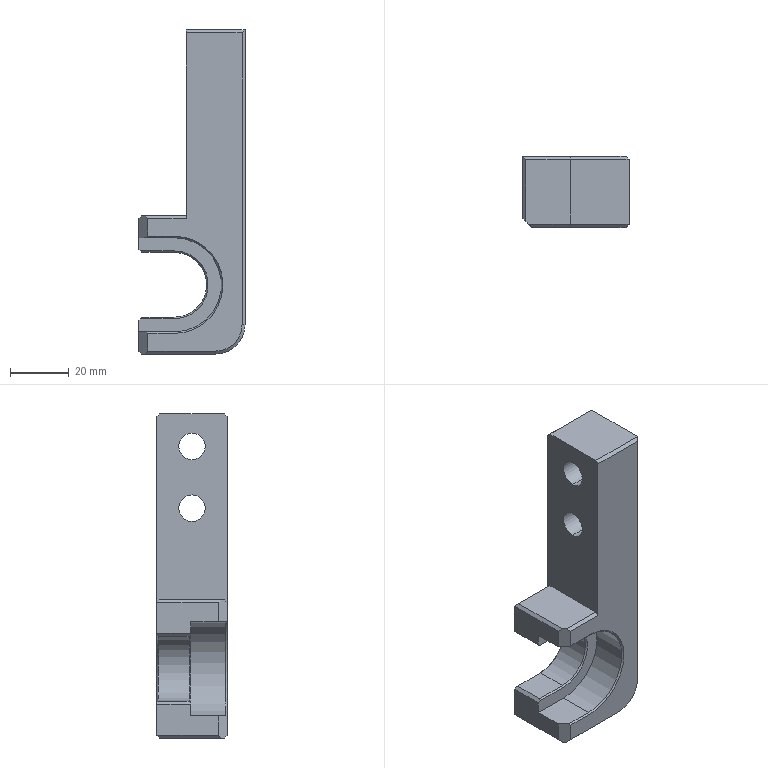Part | SolidWorks | features Chamfer 7, ICE 3, Extrusion 1, Fillet 1, HoleWzd 1 | 1 solid | 52 faces | box 36 x 24 x 110 mm | volume 50408 mm3 | plane 36 | cylinder 11 | cone 5 | commonest cylinder face diameters 9 x4 15 x4 20 x1 22 x1 32 x1
STEP:
#1=CARTESIAN_POINT('',(1.,0.,325.519));
#2=VERTEX_POINT('',#1);
#3=CARTESIAN_POINT('',(1.,0.,310.519));
#4=VERTEX_POINT('',#3);
#5=CARTESIAN_POINT('',(1.,0.,318.019));
#6=DIRECTION('',(1.,0.,0.));
#7=DIRECTION('',(0.,0.,-1.));
#8=AXIS2_PLACEMENT_3D('',#5,#6,#7);
#9=CIRCLE('',#8,7.5);
#10=EDGE_CURVE('',#2,#4,#9,.T.);
#11=ORIENTED_EDGE('',*,*,#10,.F.);
#12=CARTESIAN_POINT('',(10.,0.,325.519));
#13=VERTEX_POINT('',#12);
#14=CARTESIAN_POINT('',(10.,0.,325.519));
#15=DIRECTION('',(1.,0.,0.));
#16=VECTOR('',#15,1000.);
#17=LINE('',#14,#16);
#18=EDGE_CURVE('',#2,#13,#17,.T.);
#19=ORIENTED_EDGE('',*,*,#18,.T.);
#20=CARTESIAN_POINT('',(10.,0.,310.519));
#21=VERTEX_POINT('',#20);
#22=CARTESIAN_POINT('',(10.,0.,318.019));
#23=DIRECTION('',(1.,0.,0.));
#24=DIRECTION('',(0.,0.,-1.));
#25=AXIS2_PLACEMENT_3D('',#22,#23,#24);
#26=CIRCLE('',#25,7.5);
#27=EDGE_CURVE('',#13,#21,#26,.T.);
#28=ORIENTED_EDGE('',*,*,#27,.T.);
#29=CARTESIAN_POINT('',(10.,0.,310.519));
#30=DIRECTION('',(1.,0.,0.));
#31=VECTOR('',#30,1000.);
#32=LINE('',#29,#31);
#33=EDGE_CURVE('',#4,#21,#32,.T.);
#34=ORIENTED_EDGE('',*,*,#33,.F.);
#35=EDGE_LOOP('',(#11,#19,#28,#34));
#36=FACE_OUTER_BOUND('',#35,.T.);
#37=CARTESIAN_POINT('',(10.,0.,318.019));
#38=DIRECTION('',(1.,0.,0.));
#39=DIRECTION('',(0.,0.,-1.));
#40=AXIS2_PLACEMENT_3D('',#37,#38,#39);
#41=CYLINDRICAL_SURFACE('',#40,7.5);
#42=ADVANCED_FACE('',(#36),#41,.F.);
#43=CARTESIAN_POINT('',(-10.,0.,322.519));
#44=VERTEX_POINT('',#43);
#45=CARTESIAN_POINT('',(-10.,0.,313.519));
#46=VERTEX_POINT('',#45);
#47=CARTESIAN_POINT('',(-10.,0.,318.019));
#48=DIRECTION('',(1.,0.,0.));
#49=DIRECTION('',(0.,1.,0.));
#50=AXIS2_PLACEMENT_3D('',#47,#48,#49);
#51=CIRCLE('',#50,4.5);
#52=EDGE_CURVE('',#44,#46,#51,.T.);
#53=ORIENTED_EDGE('',*,*,#52,.F.);
#54=CARTESIAN_POINT('',(1.,0.,322.519));
#55=VERTEX_POINT('',#54);
#56=CARTESIAN_POINT('',(10.,0.,322.519));
#57=DIRECTION('',(1.,0.,0.));
#58=VECTOR('',#57,1000.);
#59=LINE('',#56,#58);
#60=EDGE_CURVE('',#44,#55,#59,.T.);
#61=ORIENTED_EDGE('',*,*,#60,.T.);
#62=CARTESIAN_POINT('',(1.,0.,313.519));
#63=VERTEX_POINT('',#62);
#64=CARTESIAN_POINT('',(1.,0.,318.019));
#65=DIRECTION('',(1.,0.,0.));
#66=DIRECTION('',(0.,0.,-1.));
#67=AXIS2_PLACEMENT_3D('',#64,#65,#66);
#68=CIRCLE('',#67,4.5);
#69=EDGE_CURVE('',#55,#63,#68,.T.);
#70=ORIENTED_EDGE('',*,*,#69,.T.);
#71=CARTESIAN_POINT('',(10.,0.,313.519));
#72=DIRECTION('',(1.,0.,0.));
#73=VECTOR('',#72,1000.);
#74=LINE('',#71,#73);
#75=EDGE_CURVE('',#46,#63,#74,.T.);
#76=ORIENTED_EDGE('',*,*,#75,.F.);
#77=EDGE_LOOP('',(#53,#61,#70,#76));
#78=FACE_OUTER_BOUND('',#77,.T.);
#79=CARTESIAN_POINT('',(10.,0.,318.019));
#80=DIRECTION('',(1.,0.,0.));
#81=DIRECTION('',(0.,0.,-1.));
#82=AXIS2_PLACEMENT_3D('',#79,#80,#81);
#83=CYLINDRICAL_SURFACE('',#82,4.5);
#84=ADVANCED_FACE('',(#78),#83,.F.);
#85=CARTESIAN_POINT('',(1.,0.,304.519));
#86=VERTEX_POINT('',#85);
#87=CARTESIAN_POINT('',(1.,0.,289.519));
#88=VERTEX_POINT('',#87);
#89=CARTESIAN_POINT('',(1.,0.,297.019));
#90=DIRECTION('',(1.,0.,0.));
#91=DIRECTION('',(0.,0.,-1.));
#92=AXIS2_PLACEMENT_3D('',#89,#90,#91);
#93=CIRCLE('',#92,7.5);
#94=EDGE_CURVE('',#86,#88,#93,.T.);
#95=ORIENTED_EDGE('',*,*,#94,.F.);
#96=CARTESIAN_POINT('',(10.,0.,304.519));
#97=VERTEX_POINT('',#96);
#98=CARTESIAN_POINT('',(10.,0.,304.519));
#99=DIRECTION('',(1.,0.,0.));
#100=VECTOR('',#99,1000.);
#101=LINE('',#98,#100);
#102=EDGE_CURVE('',#86,#97,#101,.T.);
#103=ORIENTED_EDGE('',*,*,#102,.T.);
#104=CARTESIAN_POINT('',(10.,0.,289.519));
#105=VERTEX_POINT('',#104);
#106=CARTESIAN_POINT('',(10.,0.,297.019));
#107=DIRECTION('',(1.,0.,0.));
#108=DIRECTION('',(0.,0.,-1.));
#109=AXIS2_PLACEMENT_3D('',#106,#107,#108);
#110=CIRCLE('',#109,7.5);
#111=EDGE_CURVE('',#97,#105,#110,.T.);
#112=ORIENTED_EDGE('',*,*,#111,.T.);
#113=CARTESIAN_POINT('',(10.,0.,289.519));
#114=DIRECTION('',(1.,0.,0.));
#115=VECTOR('',#114,1000.);
#116=LINE('',#113,#115);
#117=EDGE_CURVE('',#88,#105,#116,.T.);
#118=ORIENTED_EDGE('',*,*,#117,.F.);
#119=EDGE_LOOP('',(#95,#103,#112,#118));
#120=FACE_OUTER_BOUND('',#119,.T.);
#121=CARTESIAN_POINT('',(10.,0.,297.019));
#122=DIRECTION('',(1.,0.,0.));
#123=DIRECTION('',(0.,0.,-1.));
#124=AXIS2_PLACEMENT_3D('',#121,#122,#123);
#125=CYLINDRICAL_SURFACE('',#124,7.5);
#126=ADVANCED_FACE('',(#120),#125,.F.);
#127=CARTESIAN_POINT('',(-10.,0.,301.519));
#128=VERTEX_POINT('',#127);
#129=CARTESIAN_POINT('',(-10.,0.,292.519));
#130=VERTEX_POINT('',#129);
#131=CARTESIAN_POINT('',(-10.,0.,297.019));
#132=DIRECTION('',(1.,0.,0.));
#133=DIRECTION('',(0.,1.,0.));
#134=AXIS2_PLACEMENT_3D('',#131,#132,#133);
#135=CIRCLE('',#134,4.5);
#136=EDGE_CURVE('',#128,#130,#135,.T.);
#137=ORIENTED_EDGE('',*,*,#136,.F.);
#138=CARTESIAN_POINT('',(1.,0.,301.519));
#139=VERTEX_POINT('',#138);
#140=CARTESIAN_POINT('',(10.,0.,301.519));
#141=DIRECTION('',(1.,0.,0.));
#142=VECTOR('',#141,1000.);
#143=LINE('',#140,#142);
#144=EDGE_CURVE('',#128,#139,#143,.T.);
#145=ORIENTED_EDGE('',*,*,#144,.T.);
#146=CARTESIAN_POINT('',(1.,0.,292.519));
#147=VERTEX_POINT('',#146);
#148=CARTESIAN_POINT('',(1.,0.,297.019));
#149=DIRECTION('',(1.,0.,0.));
#150=DIRECTION('',(0.,0.,-1.));
#151=AXIS2_PLACEMENT_3D('',#148,#149,#150);
#152=CIRCLE('',#151,4.5);
#153=EDGE_CURVE('',#139,#147,#152,.T.);
#154=ORIENTED_EDGE('',*,*,#153,.T.);
#155=CARTESIAN_POINT('',(10.,0.,292.519));
#156=DIRECTION('',(1.,0.,0.));
#157=VECTOR('',#156,1000.);
#158=LINE('',#155,#157);
#159=EDGE_CURVE('',#130,#147,#158,.T.);
#160=ORIENTED_EDGE('',*,*,#159,.F.);
#161=EDGE_LOOP('',(#137,#145,#154,#160));
#162=FACE_OUTER_BOUND('',#161,.T.);
#163=CARTESIAN_POINT('',(10.,0.,297.019));
#164=DIRECTION('',(1.,0.,0.));
#165=DIRECTION('',(0.,0.,-1.));
#166=AXIS2_PLACEMENT_3D('',#163,#164,#165);
#167=CYLINDRICAL_SURFACE('',#166,4.5);
#168=ADVANCED_FACE('',(#162),#167,.F.);
#169=CARTESIAN_POINT('',(-26.,-9.,258.519));
#170=VERTEX_POINT('',#169);
#171=CARTESIAN_POINT('',(-26.,0.5,258.519));
#172=VERTEX_POINT('',#171);
#173=CARTESIAN_POINT('',(-26.,0.,258.519));
#174=DIRECTION('',(0.,1.,0.));
#175=VECTOR('',#174,1000.);
#176=LINE('',#173,#175);
#177=EDGE_CURVE('',#170,#172,#176,.T.);
#178=ORIENTED_EDGE('',*,*,#177,.F.);
#179=CARTESIAN_POINT('',(-26.,-9.,265.019));
#180=VERTEX_POINT('',#179);
#181=CARTESIAN_POINT('',(-26.,-9.,0.));
#182=DIRECTION('',(0.,0.,1.));
#183=VECTOR('',#182,1000.);
#184=LINE('',#181,#183);
#185=EDGE_CURVE('',#170,#180,#184,.T.);
#186=ORIENTED_EDGE('',*,*,#185,.T.);
#187=CARTESIAN_POINT('',(-26.,12.,265.019));
#188=VERTEX_POINT('',#187);
#189=CARTESIAN_POINT('',(-26.,0.,265.019));
#190=DIRECTION('',(0.,1.,0.));
#191=VECTOR('',#190,1000.);
#192=LINE('',#189,#191);
#193=EDGE_CURVE('',#180,#188,#192,.T.);
#194=ORIENTED_EDGE('',*,*,#193,.T.);
#195=CARTESIAN_POINT('',(-26.,12.,254.519));
#196=VERTEX_POINT('',#195);
#197=CARTESIAN_POINT('',(-26.,12.,219.019));
#198=DIRECTION('',(0.,0.,-1.));
#199=VECTOR('',#198,1000.);
#200=LINE('',#197,#199);
#201=EDGE_CURVE('',#188,#196,#200,.T.);
#202=ORIENTED_EDGE('',*,*,#201,.T.);
#203=CARTESIAN_POINT('',(-26.,0.5,254.519));
#204=VERTEX_POINT('',#203);
#205=CARTESIAN_POINT('',(-26.,0.,254.519));
#206=DIRECTION('',(0.,-1.,0.));
#207=VECTOR('',#206,1000.);
#208=LINE('',#205,#207);
#209=EDGE_CURVE('',#196,#204,#208,.T.);
#210=ORIENTED_EDGE('',*,*,#209,.T.);
#211=CARTESIAN_POINT('',(-26.,0.5,0.));
#212=DIRECTION('',(0.,0.,1.));
#213=VECTOR('',#212,1000.);
#214=LINE('',#211,#213);
#215=EDGE_CURVE('',#204,#172,#214,.T.);
#216=ORIENTED_EDGE('',*,*,#215,.T.);
#217=EDGE_LOOP('',(#178,#186,#194,#202,#210,#216));
#218=FACE_OUTER_BOUND('',#217,.T.);
#219=CARTESIAN_POINT('',(-26.,0.,0.));
#220=DIRECTION('',(1.,0.,0.));
#221=DIRECTION('',(0.,1.,0.));
#222=AXIS2_PLACEMENT_3D('',#219,#220,#221);
#223=PLANE('',#222);
#224=ADVANCED_FACE('',(#218),#223,.F.);
#225=CARTESIAN_POINT('',(-14.,-12.,226.019));
#226=VERTEX_POINT('',#225);
#227=CARTESIAN_POINT('',(-23.,-12.,226.019));
#228=VERTEX_POINT('',#227);
#229=CARTESIAN_POINT('',(-26.,-12.,226.019));
#230=DIRECTION('',(-1.,0.,0.));
#231=VECTOR('',#230,1000.);
#232=LINE('',#229,#231);
#233=EDGE_CURVE('',#226,#228,#232,.T.);
#234=ORIENTED_EDGE('',*,*,#233,.T.);
#235=CARTESIAN_POINT('',(-23.,-12.,220.019));
#236=VERTEX_POINT('',#235);
#237=CARTESIAN_POINT('',(-23.,-12.,329.019));
#238=DIRECTION('',(0.,0.,-1.));
#239=VECTOR('',#238,1000.);
#240=LINE('',#237,#239);
#241=EDGE_CURVE('',#228,#236,#240,.T.);
#242=ORIENTED_EDGE('',*,*,#241,.T.);
#243=CARTESIAN_POINT('',(0.,-12.,220.019));
#244=VERTEX_POINT('',#243);
#245=CARTESIAN_POINT('',(-10.,-12.,220.019));
#246=DIRECTION('',(1.,0.,0.));
#247=VECTOR('',#246,1000.);
#248=LINE('',#245,#247);
#249=EDGE_CURVE('',#236,#244,#248,.T.);
#250=ORIENTED_EDGE('',*,*,#249,.T.);
#251=CARTESIAN_POINT('',(9.,-12.,229.019));
#252=VERTEX_POINT('',#251);
#253=CARTESIAN_POINT('',(0.,-12.,229.019));
#254=DIRECTION('',(0.,-1.,0.));
#255=DIRECTION('',(0.,0.,1.));
#256=AXIS2_PLACEMENT_3D('',#253,#254,#255);
#257=CIRCLE('',#256,9.);
#258=EDGE_CURVE('',#244,#252,#257,.T.);
#259=ORIENTED_EDGE('',*,*,#258,.T.);
#260=CARTESIAN_POINT('',(9.,-12.,328.019));
#261=VERTEX_POINT('',#260);
#262=CARTESIAN_POINT('',(9.,-12.,329.019));
#263=DIRECTION('',(0.,0.,1.));
#264=VECTOR('',#263,1000.);
#265=LINE('',#262,#264);
#266=EDGE_CURVE('',#252,#261,#265,.T.);
#267=ORIENTED_EDGE('',*,*,#266,.T.);
#268=CARTESIAN_POINT('',(-10.,-12.,328.019));
#269=VERTEX_POINT('',#268);
#270=CARTESIAN_POINT('',(-10.,-12.,328.019));
#271=DIRECTION('',(-1.,0.,0.));
#272=VECTOR('',#271,1000.);
#273=LINE('',#270,#272);
#274=EDGE_CURVE('',#261,#269,#273,.T.);
#275=ORIENTED_EDGE('',*,*,#274,.T.);
#276=CARTESIAN_POINT('',(-10.,-12.,265.019));
#277=VERTEX_POINT('',#276);
#278=CARTESIAN_POINT('',(-10.,-12.,329.019));
#279=DIRECTION('',(0.,0.,-1.));
#280=VECTOR('',#279,1000.);
#281=LINE('',#278,#280);
#282=EDGE_CURVE('',#269,#277,#281,.T.);
#283=ORIENTED_EDGE('',*,*,#282,.T.);
#284=CARTESIAN_POINT('',(-23.,-12.,265.019));
#285=VERTEX_POINT('',#284);
#286=CARTESIAN_POINT('',(-10.,-12.,265.019));
#287=DIRECTION('',(-1.,0.,0.));
#288=VECTOR('',#287,1000.);
#289=LINE('',#286,#288);
#290=EDGE_CURVE('',#277,#285,#289,.T.);
#291=ORIENTED_EDGE('',*,*,#290,.T.);
#292=CARTESIAN_POINT('',(-23.,-12.,259.019));
#293=VERTEX_POINT('',#292);
#294=CARTESIAN_POINT('',(-23.,-12.,329.019));
#295=DIRECTION('',(0.,0.,-1.));
#296=VECTOR('',#295,1000.);
#297=LINE('',#294,#296);
#298=EDGE_CURVE('',#285,#293,#297,.T.);
#299=ORIENTED_EDGE('',*,*,#298,.T.);
#300=CARTESIAN_POINT('',(-14.,-12.,259.019));
#301=VERTEX_POINT('',#300);
#302=CARTESIAN_POINT('',(-14.,-12.,259.019));
#303=DIRECTION('',(1.,0.,0.));
#304=VECTOR('',#303,1000.);
#305=LINE('',#302,#304);
#306=EDGE_CURVE('',#293,#301,#305,.T.);
#307=ORIENTED_EDGE('',*,*,#306,.T.);
#308=CARTESIAN_POINT('',(-14.,-12.,242.519));
#309=DIRECTION('',(0.,1.,0.));
#310=DIRECTION('',(0.,0.,1.));
#311=AXIS2_PLACEMENT_3D('',#308,#309,#310);
#312=CIRCLE('',#311,16.5);
#313=EDGE_CURVE('',#301,#226,#312,.T.);
#314=ORIENTED_EDGE('',*,*,#313,.T.);
#315=EDGE_LOOP('',(#234,#242,#250,#259,#267,#275,#283,#291,#299,#307,#314));
#316=FACE_OUTER_BOUND('',#315,.T.);
#317=CARTESIAN_POINT('',(-10.,-12.,329.019));
#318=DIRECTION('',(0.,1.,0.));
#319=DIRECTION('',(0.,0.,1.));
#320=AXIS2_PLACEMENT_3D('',#317,#318,#319);
#321=PLANE('',#320);
#322=ADVANCED_FACE('',(#316),#321,.F.);
#323=CARTESIAN_POINT('',(-26.,12.,220.019));
#324=VERTEX_POINT('',#323);
#325=CARTESIAN_POINT('',(-26.,-9.,220.019));
#326=VERTEX_POINT('',#325);
#327=CARTESIAN_POINT('',(-26.,0.,220.019));
#328=DIRECTION('',(0.,-1.,0.));
#329=VECTOR('',#328,1000.);
#330=LINE('',#327,#329);
#331=EDGE_CURVE('',#324,#326,#330,.T.);
#332=ORIENTED_EDGE('',*,*,#331,.T.);
#333=CARTESIAN_POINT('',(-26.,-9.,226.519));
#334=VERTEX_POINT('',#333);
#335=CARTESIAN_POINT('',(-26.,-9.,0.));
#336=DIRECTION('',(0.,0.,1.));
#337=VECTOR('',#336,1000.);
#338=LINE('',#335,#337);
#339=EDGE_CURVE('',#326,#334,#338,.T.);
#340=ORIENTED_EDGE('',*,*,#339,.T.);
#341=CARTESIAN_POINT('',(-26.,0.5,226.519));
#342=VERTEX_POINT('',#341);
#343=CARTESIAN_POINT('',(-26.,0.,226.519));
#344=DIRECTION('',(0.,-1.,0.));
#345=VECTOR('',#344,1000.);
#346=LINE('',#343,#345);
#347=EDGE_CURVE('',#342,#334,#346,.T.);
#348=ORIENTED_EDGE('',*,*,#347,.F.);
#349=CARTESIAN_POINT('',(-26.,0.5,230.519));
#350=VERTEX_POINT('',#349);
#351=CARTESIAN_POINT('',(-26.,0.5,0.));
#352=DIRECTION('',(0.,0.,1.));
#353=VECTOR('',#352,1000.);
#354=LINE('',#351,#353);
#355=EDGE_CURVE('',#342,#350,#354,.T.);
#356=ORIENTED_EDGE('',*,*,#355,.T.);
#357=CARTESIAN_POINT('',(-26.,12.,230.519));
#358=VERTEX_POINT('',#357);
#359=CARTESIAN_POINT('',(-26.,0.,230.519));
#360=DIRECTION('',(0.,1.,0.));
#361=VECTOR('',#360,1000.);
#362=LINE('',#359,#361);
#363=EDGE_CURVE('',#350,#358,#362,.T.);
#364=ORIENTED_EDGE('',*,*,#363,.T.);
#365=CARTESIAN_POINT('',(-26.,12.,219.019));
#366=DIRECTION('',(0.,0.,-1.));
#367=VECTOR('',#366,1000.);
#368=LINE('',#365,#367);
#369=EDGE_CURVE('',#358,#324,#368,.T.);
#370=ORIENTED_EDGE('',*,*,#369,.T.);
#371=EDGE_LOOP('',(#332,#340,#348,#356,#364,#370));
#372=FACE_OUTER_BOUND('',#371,.T.);
#373=CARTESIAN_POINT('',(-26.,0.,0.));
#374=DIRECTION('',(1.,0.,0.));
#375=DIRECTION('',(0.,1.,0.));
#376=AXIS2_PLACEMENT_3D('',#373,#374,#375);
#377=PLANE('',#376);
#378=ADVANCED_FACE('',(#372),#377,.F.);
#379=CARTESIAN_POINT('',(-10.,0.,318.019));
#380=DIRECTION('',(1.,0.,0.));
#381=DIRECTION('',(0.,1.,0.));
#382=AXIS2_PLACEMENT_3D('',#379,#380,#381);
#383=CIRCLE('',#382,4.5);
#384=EDGE_CURVE('',#46,#44,#383,.T.);
#385=ORIENTED_EDGE('',*,*,#384,.T.);
#386=ORIENTED_EDGE('',*,*,#52,.T.);
#387=EDGE_LOOP('',(#385,#386));
#388=FACE_BOUND('',#387,.T.);
#389=CARTESIAN_POINT('',(-10.,0.,297.019));
#390=DIRECTION('',(1.,0.,0.));
#391=DIRECTION('',(0.,1.,0.));
#392=AXIS2_PLACEMENT_3D('',#389,#390,#391);
#393=CIRCLE('',#392,4.5);
#394=EDGE_CURVE('',#130,#128,#393,.T.);
#395=ORIENTED_EDGE('',*,*,#394,.T.);
#396=ORIENTED_EDGE('',*,*,#136,.T.);
#397=EDGE_LOOP('',(#395,#396));
#398=FACE_BOUND('',#397,.T.);
#399=CARTESIAN_POINT('',(-10.,11.,329.019));
#400=VERTEX_POINT('',#399);
#401=CARTESIAN_POINT('',(-10.,-11.,329.019));
#402=VERTEX_POINT('',#401);
#403=CARTESIAN_POINT('',(-10.,12.,329.019));
#404=DIRECTION('',(0.,-1.,0.));
#405=VECTOR('',#404,1000.);
#406=LINE('',#403,#405);
#407=EDGE_CURVE('',#400,#402,#406,.T.);
#408=ORIENTED_EDGE('',*,*,#407,.F.);
#409=CARTESIAN_POINT('',(-10.,12.,328.019));
#410=VERTEX_POINT('',#409);
#411=CARTESIAN_POINT('',(-10.,11.,329.019));
#412=DIRECTION('',(0.,0.7071,-0.7071));
#413=VECTOR('',#412,1000.);
#414=LINE('',#411,#413);
#415=EDGE_CURVE('',#400,#410,#414,.T.);
#416=ORIENTED_EDGE('',*,*,#415,.T.);
#417=CARTESIAN_POINT('',(-10.,12.,265.019));
#418=VERTEX_POINT('',#417);
#419=CARTESIAN_POINT('',(-10.,12.,329.019));
#420=DIRECTION('',(0.,0.,-1.));
#421=VECTOR('',#420,1000.);
#422=LINE('',#419,#421);
#423=EDGE_CURVE('',#410,#418,#422,.T.);
#424=ORIENTED_EDGE('',*,*,#423,.T.);
#425=CARTESIAN_POINT('',(-10.,11.,266.019));
#426=VERTEX_POINT('',#425);
#427=CARTESIAN_POINT('',(-10.,-20.,297.019));
#428=DIRECTION('',(0.,-0.7071,0.7071));
#429=VECTOR('',#428,1000.);
#430=LINE('',#427,#429);
#431=EDGE_CURVE('',#418,#426,#430,.T.);
#432=ORIENTED_EDGE('',*,*,#431,.T.);
#433=CARTESIAN_POINT('',(-10.,-11.,266.019));
#434=VERTEX_POINT('',#433);
#435=CARTESIAN_POINT('',(-10.,-12.,266.019));
#436=DIRECTION('',(0.,1.,0.));
#437=VECTOR('',#436,1000.);
#438=LINE('',#435,#437);
#439=EDGE_CURVE('',#434,#426,#438,.T.);
#440=ORIENTED_EDGE('',*,*,#439,.F.);
#441=CARTESIAN_POINT('',(-10.,32.,309.019));
#442=DIRECTION('',(0.,-0.7071,-0.7071));
#443=VECTOR('',#442,1000.);
#444=LINE('',#441,#443);
#445=EDGE_CURVE('',#434,#277,#444,.T.);
#446=ORIENTED_EDGE('',*,*,#445,.T.);
#447=ORIENTED_EDGE('',*,*,#282,.F.);
#448=CARTESIAN_POINT('',(-10.,-11.,329.019));
#449=DIRECTION('',(0.,0.7071,0.7071));
#450=VECTOR('',#449,1000.);
#451=LINE('',#448,#450);
#452=EDGE_CURVE('',#269,#402,#451,.T.);
#453=ORIENTED_EDGE('',*,*,#452,.T.);
#454=EDGE_LOOP('',(#408,#416,#424,#432,#440,#446,#447,#453));
#455=FACE_OUTER_BOUND('',#454,.T.);
#456=CARTESIAN_POINT('',(-10.,12.,329.019));
#457=DIRECTION('',(1.,0.,0.));
#458=DIRECTION('',(0.,1.,0.));
#459=AXIS2_PLACEMENT_3D('',#456,#457,#458);
#460=PLANE('',#459);
#461=ADVANCED_FACE('',(#388,#398,#455),#460,.F.);
#462=CARTESIAN_POINT('',(10.,0.,318.019));
#463=DIRECTION('',(1.,0.,0.));
#464=DIRECTION('',(0.,0.,-1.));
#465=AXIS2_PLACEMENT_3D('',#462,#463,#464);
#466=CIRCLE('',#465,7.5);
#467=EDGE_CURVE('',#21,#13,#466,.T.);
#468=ORIENTED_EDGE('',*,*,#467,.F.);
#469=ORIENTED_EDGE('',*,*,#27,.F.);
#470=EDGE_LOOP('',(#468,#469));
#471=FACE_BOUND('',#470,.T.);
#472=CARTESIAN_POINT('',(10.,0.,297.019));
#473=DIRECTION('',(1.,0.,0.));
#474=DIRECTION('',(0.,0.,-1.));
#475=AXIS2_PLACEMENT_3D('',#472,#473,#474);
#476=CIRCLE('',#475,7.5);
#477=EDGE_CURVE('',#105,#97,#476,.T.);
#478=ORIENTED_EDGE('',*,*,#477,.F.);
#479=ORIENTED_EDGE('',*,*,#111,.F.);
#480=EDGE_LOOP('',(#478,#479));
#481=FACE_BOUND('',#480,.T.);
#482=CARTESIAN_POINT('',(10.,-11.,229.019));
#483=VERTEX_POINT('',#482);
#484=CARTESIAN_POINT('',(10.,11.,229.019));
#485=VERTEX_POINT('',#484);
#486=CARTESIAN_POINT('',(10.,12.,229.019));
#487=DIRECTION('',(0.,1.,0.));
#488=VECTOR('',#487,1000.);
#489=LINE('',#486,#488);
#490=EDGE_CURVE('',#483,#485,#489,.T.);
#491=ORIENTED_EDGE('',*,*,#490,.T.);
#492=CARTESIAN_POINT('',(10.,11.,329.019));
#493=VERTEX_POINT('',#492);
#494=CARTESIAN_POINT('',(10.,11.,329.019));
#495=DIRECTION('',(0.,0.,1.));
#496=VECTOR('',#495,1000.);
#497=LINE('',#494,#496);
#498=EDGE_CURVE('',#485,#493,#497,.T.);
#499=ORIENTED_EDGE('',*,*,#498,.T.);
#500=CARTESIAN_POINT('',(10.,-11.,329.019));
#501=VERTEX_POINT('',#500);
#502=CARTESIAN_POINT('',(10.,12.,329.019));
#503=DIRECTION('',(0.,1.,0.));
#504=VECTOR('',#503,1000.);
#505=LINE('',#502,#504);
#506=EDGE_CURVE('',#501,#493,#505,.T.);
#507=ORIENTED_EDGE('',*,*,#506,.F.);
#508=CARTESIAN_POINT('',(10.,-11.,329.019));
#509=DIRECTION('',(0.,0.,-1.));
#510=VECTOR('',#509,1000.);
#511=LINE('',#508,#510);
#512=EDGE_CURVE('',#501,#483,#511,.T.);
#513=ORIENTED_EDGE('',*,*,#512,.T.);
#514=EDGE_LOOP('',(#491,#499,#507,#513));
#515=FACE_OUTER_BOUND('',#514,.T.);
#516=CARTESIAN_POINT('',(10.,12.,329.019));
#517=DIRECTION('',(-1.,0.,0.));
#518=DIRECTION('',(0.,-1.,0.));
#519=AXIS2_PLACEMENT_3D('',#516,#517,#518);
#520=PLANE('',#519);
#521=ADVANCED_FACE('',(#471,#481,#515),#520,.F.);
#522=ORIENTED_EDGE('',*,*,#201,.F.);
#523=CARTESIAN_POINT('',(-10.,12.,265.019));
#524=DIRECTION('',(1.,0.,0.));
#525=VECTOR('',#524,1000.);
#526=LINE('',#523,#525);
#527=EDGE_CURVE('',#188,#418,#526,.T.);
#528=ORIENTED_EDGE('',*,*,#527,.T.);
#529=ORIENTED_EDGE('',*,*,#423,.F.);
#530=CARTESIAN_POINT('',(9.,12.,328.019));
#531=VERTEX_POINT('',#530);
#532=CARTESIAN_POINT('',(10.,12.,328.019));
#533=DIRECTION('',(1.,0.,0.));
#534=VECTOR('',#533,1000.);
#535=LINE('',#532,#534);
#536=EDGE_CURVE('',#410,#531,#535,.T.);
#537=ORIENTED_EDGE('',*,*,#536,.T.);
#538=CARTESIAN_POINT('',(9.,12.,229.019));
#539=VERTEX_POINT('',#538);
#540=CARTESIAN_POINT('',(9.,12.,329.019));
#541=DIRECTION('',(0.,0.,-1.));
#542=VECTOR('',#541,1000.);
#543=LINE('',#540,#542);
#544=EDGE_CURVE('',#531,#539,#543,.T.);
#545=ORIENTED_EDGE('',*,*,#544,.T.);
#546=CARTESIAN_POINT('',(0.,12.,220.019));
#547=VERTEX_POINT('',#546);
#548=CARTESIAN_POINT('',(0.,12.,229.019));
#549=DIRECTION('',(0.,1.,0.));
#550=DIRECTION('',(0.,0.,-1.));
#551=AXIS2_PLACEMENT_3D('',#548,#549,#550);
#552=CIRCLE('',#551,9.);
#553=EDGE_CURVE('',#539,#547,#552,.T.);
#554=ORIENTED_EDGE('',*,*,#553,.T.);
#555=CARTESIAN_POINT('',(-10.,12.,220.019));
#556=DIRECTION('',(-1.,0.,0.));
#557=VECTOR('',#556,1000.);
#558=LINE('',#555,#557);
#559=EDGE_CURVE('',#547,#324,#558,.T.);
#560=ORIENTED_EDGE('',*,*,#559,.T.);
#561=ORIENTED_EDGE('',*,*,#369,.F.);
#562=CARTESIAN_POINT('',(-25.5,12.,231.019));
#563=VERTEX_POINT('',#562);
#564=CARTESIAN_POINT('',(-26.,12.,230.519));
#565=DIRECTION('',(0.7071,0.,0.7071));
#566=VECTOR('',#565,1000.);
#567=LINE('',#564,#566);
#568=EDGE_CURVE('',#358,#563,#567,.T.);
#569=ORIENTED_EDGE('',*,*,#568,.T.);
#570=CARTESIAN_POINT('',(-14.,12.,231.019));
#571=VERTEX_POINT('',#570);
#572=CARTESIAN_POINT('',(-10.,12.,231.019));
#573=DIRECTION('',(1.,0.,0.));
#574=VECTOR('',#573,1000.);
#575=LINE('',#572,#574);
#576=EDGE_CURVE('',#563,#571,#575,.T.);
#577=ORIENTED_EDGE('',*,*,#576,.T.);
#578=CARTESIAN_POINT('',(-14.,12.,254.019));
#579=VERTEX_POINT('',#578);
#580=CARTESIAN_POINT('',(-14.,12.,242.519));
#581=DIRECTION('',(0.,-1.,0.));
#582=DIRECTION('',(0.,0.,-1.));
#583=AXIS2_PLACEMENT_3D('',#580,#581,#582);
#584=CIRCLE('',#583,11.5);
#585=EDGE_CURVE('',#571,#579,#584,.T.);
#586=ORIENTED_EDGE('',*,*,#585,.T.);
#587=CARTESIAN_POINT('',(-25.5,12.,254.019));
#588=VERTEX_POINT('',#587);
#589=CARTESIAN_POINT('',(-10.,12.,254.019));
#590=DIRECTION('',(-1.,0.,0.));
#591=VECTOR('',#590,1000.);
#592=LINE('',#589,#591);
#593=EDGE_CURVE('',#579,#588,#592,.T.);
#594=ORIENTED_EDGE('',*,*,#593,.T.);
#595=CARTESIAN_POINT('',(-26.,12.,254.519));
#596=DIRECTION('',(-0.7071,0.,0.7071));
#597=VECTOR('',#596,1000.);
#598=LINE('',#595,#597);
#599=EDGE_CURVE('',#588,#196,#598,.T.);
#600=ORIENTED_EDGE('',*,*,#599,.T.);
#601=EDGE_LOOP('',(#522,#528,#529,#537,#545,#554,#560,#561,#569,#577,#586,#594,#600));
#602=FACE_OUTER_BOUND('',#601,.T.);
#603=CARTESIAN_POINT('',(-10.,12.,329.019));
#604=DIRECTION('',(0.,-1.,0.));
#605=DIRECTION('',(0.,0.,-1.));
#606=AXIS2_PLACEMENT_3D('',#603,#604,#605);
#607=PLANE('',#606);
#608=ADVANCED_FACE('',(#602),#607,.F.);
#609=ORIENTED_EDGE('',*,*,#506,.T.);
#610=CARTESIAN_POINT('',(-10.,11.,329.019));
#611=DIRECTION('',(-1.,0.,0.));
#612=VECTOR('',#611,1000.);
#613=LINE('',#610,#612);
#614=EDGE_CURVE('',#493,#400,#613,.T.);
#615=ORIENTED_EDGE('',*,*,#614,.T.);
#616=ORIENTED_EDGE('',*,*,#407,.T.);
#617=CARTESIAN_POINT('',(10.,-11.,329.019));
#618=DIRECTION('',(1.,0.,0.));
#619=VECTOR('',#618,1000.);
#620=LINE('',#617,#619);
#621=EDGE_CURVE('',#402,#501,#620,.T.);
#622=ORIENTED_EDGE('',*,*,#621,.T.);
#623=EDGE_LOOP('',(#609,#615,#616,#622));
#624=FACE_OUTER_BOUND('',#623,.T.);
#625=CARTESIAN_POINT('',(10.,-12.,329.019));
#626=DIRECTION('',(0.,0.,1.));
#627=DIRECTION('',(1.,0.,0.));
#628=AXIS2_PLACEMENT_3D('',#625,#626,#627);
#629=PLANE('',#628);
#630=ADVANCED_FACE('',(#624),#629,.T.);
#631=CARTESIAN_POINT('',(0.,-11.,219.019));
#632=VERTEX_POINT('',#631);
#633=CARTESIAN_POINT('',(-24.,-11.,219.019));
#634=VERTEX_POINT('',#633);
#635=CARTESIAN_POINT('',(10.,-11.,219.019));
#636=DIRECTION('',(-1.,0.,0.));
#637=VECTOR('',#636,1000.);
#638=LINE('',#635,#637);
#639=EDGE_CURVE('',#632,#634,#638,.T.);
#640=ORIENTED_EDGE('',*,*,#639,.T.);
#641=CARTESIAN_POINT('',(-25.,-10.,219.019));
#642=VERTEX_POINT('',#641);
#643=CARTESIAN_POINT('',(-26.,-9.,219.019));
#644=DIRECTION('',(-0.7071,0.7071,0.));
#645=VECTOR('',#644,1000.);
#646=LINE('',#643,#645);
#647=EDGE_CURVE('',#634,#642,#646,.T.);
#648=ORIENTED_EDGE('',*,*,#647,.T.);
#649=CARTESIAN_POINT('',(-25.,11.,219.019));
#650=VERTEX_POINT('',#649);
#651=CARTESIAN_POINT('',(-25.,-12.,219.019));
#652=DIRECTION('',(0.,1.,0.));
#653=VECTOR('',#652,1000.);
#654=LINE('',#651,#653);
#655=EDGE_CURVE('',#642,#650,#654,.T.);
#656=ORIENTED_EDGE('',*,*,#655,.T.);
#657=CARTESIAN_POINT('',(0.,11.,219.019));
#658=VERTEX_POINT('',#657);
#659=CARTESIAN_POINT('',(10.,11.,219.019));
#660=DIRECTION('',(1.,0.,0.));
#661=VECTOR('',#660,1000.);
#662=LINE('',#659,#661);
#663=EDGE_CURVE('',#650,#658,#662,.T.);
#664=ORIENTED_EDGE('',*,*,#663,.T.);
#665=CARTESIAN_POINT('',(0.,-12.,219.019));
#666=DIRECTION('',(0.,-1.,0.));
#667=VECTOR('',#666,1000.);
#668=LINE('',#665,#667);
#669=EDGE_CURVE('',#658,#632,#668,.T.);
#670=ORIENTED_EDGE('',*,*,#669,.T.);
#671=EDGE_LOOP('',(#640,#648,#656,#664,#670));
#672=FACE_OUTER_BOUND('',#671,.T.);
#673=CARTESIAN_POINT('',(10.,-12.,219.019));
#674=DIRECTION('',(0.,0.,1.));
#675=DIRECTION('',(1.,0.,0.));
#676=AXIS2_PLACEMENT_3D('',#673,#674,#675);
#677=PLANE('',#676);
#678=ADVANCED_FACE('',(#672),#677,.F.);
#679=CARTESIAN_POINT('',(-25.,11.,266.019));
#680=VERTEX_POINT('',#679);
#681=CARTESIAN_POINT('',(-25.,-10.,266.019));
#682=VERTEX_POINT('',#681);
#683=CARTESIAN_POINT('',(-25.,-12.,266.019));
#684=DIRECTION('',(0.,-1.,0.));
#685=VECTOR('',#684,1000.);
#686=LINE('',#683,#685);
#687=EDGE_CURVE('',#680,#682,#686,.T.);
#688=ORIENTED_EDGE('',*,*,#687,.T.);
#689=CARTESIAN_POINT('',(-24.,-11.,266.019));
#690=VERTEX_POINT('',#689);
#691=CARTESIAN_POINT('',(-26.,-9.,266.019));
#692=DIRECTION('',(0.7071,-0.7071,0.));
#693=VECTOR('',#692,1000.);
#694=LINE('',#691,#693);
#695=EDGE_CURVE('',#682,#690,#694,.T.);
#696=ORIENTED_EDGE('',*,*,#695,.T.);
#697=CARTESIAN_POINT('',(-26.,-11.,266.019));
#698=DIRECTION('',(1.,0.,0.));
#699=VECTOR('',#698,1000.);
#700=LINE('',#697,#699);
#701=EDGE_CURVE('',#690,#434,#700,.T.);
#702=ORIENTED_EDGE('',*,*,#701,.T.);
#703=ORIENTED_EDGE('',*,*,#439,.T.);
#704=CARTESIAN_POINT('',(-26.,11.,266.019));
#705=DIRECTION('',(-1.,0.,0.));
#706=VECTOR('',#705,1000.);
#707=LINE('',#704,#706);
#708=EDGE_CURVE('',#426,#680,#707,.T.);
#709=ORIENTED_EDGE('',*,*,#708,.T.);
#710=EDGE_LOOP('',(#688,#696,#702,#703,#709));
#711=FACE_OUTER_BOUND('',#710,.T.);
#712=CARTESIAN_POINT('',(-26.,-12.,266.019));
#713=DIRECTION('',(0.,0.,-1.));
#714=DIRECTION('',(-1.,0.,0.));
#715=AXIS2_PLACEMENT_3D('',#712,#713,#714);
#716=PLANE('',#715);
#717=ADVANCED_FACE('',(#711),#716,.F.);
#718=CARTESIAN_POINT('',(-14.,11.5,231.519));
#719=VERTEX_POINT('',#718);
#720=CARTESIAN_POINT('',(-14.,1.,231.519));
#721=VERTEX_POINT('',#720);
#722=CARTESIAN_POINT('',(-14.,18.,231.519));
#723=DIRECTION('',(0.,-1.,0.));
#724=VECTOR('',#723,1000.);
#725=LINE('',#722,#724);
#726=EDGE_CURVE('',#719,#721,#725,.T.);
#727=ORIENTED_EDGE('',*,*,#726,.T.);
#728=CARTESIAN_POINT('',(-14.,1.,253.519));
#729=VERTEX_POINT('',#728);
#730=CARTESIAN_POINT('',(-14.,1.,242.519));
#731=DIRECTION('',(0.,-1.,0.));
#732=DIRECTION('',(0.,0.,1.));
#733=AXIS2_PLACEMENT_3D('',#730,#731,#732);
#734=CIRCLE('',#733,11.);
#735=EDGE_CURVE('',#721,#729,#734,.T.);
#736=ORIENTED_EDGE('',*,*,#735,.T.);
#737=CARTESIAN_POINT('',(-14.,11.5,253.519));
#738=VERTEX_POINT('',#737);
#739=CARTESIAN_POINT('',(-14.,18.,253.519));
#740=DIRECTION('',(0.,-1.,0.));
#741=VECTOR('',#740,1000.);
#742=LINE('',#739,#741);
#743=EDGE_CURVE('',#738,#729,#742,.T.);
#744=ORIENTED_EDGE('',*,*,#743,.F.);
#745=CARTESIAN_POINT('',(-14.,11.5,242.519));
#746=DIRECTION('',(0.,1.,0.));
#747=DIRECTION('',(0.,0.,-1.));
#748=AXIS2_PLACEMENT_3D('',#745,#746,#747);
#749=CIRCLE('',#748,11.);
#750=EDGE_CURVE('',#738,#719,#749,.T.);
#751=ORIENTED_EDGE('',*,*,#750,.T.);
#752=EDGE_LOOP('',(#727,#736,#744,#751));
#753=FACE_OUTER_BOUND('',#752,.T.);
#754=CARTESIAN_POINT('',(-14.,18.,242.519));
#755=DIRECTION('',(0.,-1.,0.));
#756=DIRECTION('',(0.,0.,-1.));
#757=AXIS2_PLACEMENT_3D('',#754,#755,#756);
#758=CYLINDRICAL_SURFACE('',#757,11.);
#759=ADVANCED_FACE('',(#753),#758,.F.);
#760=CARTESIAN_POINT('',(-25.,1.,253.519));
#761=VERTEX_POINT('',#760);
#762=CARTESIAN_POINT('',(-54.,1.,253.519));
#763=DIRECTION('',(-1.,0.,0.));
#764=VECTOR('',#763,1000.);
#765=LINE('',#762,#764);
#766=EDGE_CURVE('',#729,#761,#765,.T.);
#767=ORIENTED_EDGE('',*,*,#766,.T.);
#768=CARTESIAN_POINT('',(-25.,11.5,253.519));
#769=VERTEX_POINT('',#768);
#770=CARTESIAN_POINT('',(-25.,18.,253.519));
#771=DIRECTION('',(0.,1.,0.));
#772=VECTOR('',#771,1000.);
#773=LINE('',#770,#772);
#774=EDGE_CURVE('',#761,#769,#773,.T.);
#775=ORIENTED_EDGE('',*,*,#774,.T.);
#776=CARTESIAN_POINT('',(-54.,11.5,253.519));
#777=DIRECTION('',(1.,0.,0.));
#778=VECTOR('',#777,1000.);
#779=LINE('',#776,#778);
#780=EDGE_CURVE('',#769,#738,#779,.T.);
#781=ORIENTED_EDGE('',*,*,#780,.T.);
#782=ORIENTED_EDGE('',*,*,#743,.T.);
#783=EDGE_LOOP('',(#767,#775,#781,#782));
#784=FACE_OUTER_BOUND('',#783,.T.);
#785=CARTESIAN_POINT('',(-54.,18.,253.519));
#786=DIRECTION('',(0.,0.,1.));
#787=DIRECTION('',(1.,0.,0.));
#788=AXIS2_PLACEMENT_3D('',#785,#786,#787);
#789=PLANE('',#788);
#790=ADVANCED_FACE('',(#784),#789,.F.);
#791=CARTESIAN_POINT('',(-25.,11.5,231.519));
#792=VERTEX_POINT('',#791);
#793=CARTESIAN_POINT('',(-54.,11.5,231.519));
#794=DIRECTION('',(-1.,0.,0.));
#795=VECTOR('',#794,1000.);
#796=LINE('',#793,#795);
#797=EDGE_CURVE('',#719,#792,#796,.T.);
#798=ORIENTED_EDGE('',*,*,#797,.T.);
#799=CARTESIAN_POINT('',(-25.,1.,231.519));
#800=VERTEX_POINT('',#799);
#801=CARTESIAN_POINT('',(-25.,18.,231.519));
#802=DIRECTION('',(0.,-1.,0.));
#803=VECTOR('',#802,1000.);
#804=LINE('',#801,#803);
#805=EDGE_CURVE('',#792,#800,#804,.T.);
#806=ORIENTED_EDGE('',*,*,#805,.T.);
#807=CARTESIAN_POINT('',(-54.,1.,231.519));
#808=DIRECTION('',(1.,0.,0.));
#809=VECTOR('',#808,1000.);
#810=LINE('',#807,#809);
#811=EDGE_CURVE('',#800,#721,#810,.T.);
#812=ORIENTED_EDGE('',*,*,#811,.T.);
#813=ORIENTED_EDGE('',*,*,#726,.F.);
#814=EDGE_LOOP('',(#798,#806,#812,#813));
#815=FACE_OUTER_BOUND('',#814,.T.);
#816=CARTESIAN_POINT('',(-54.,18.,231.519));
#817=DIRECTION('',(0.,0.,-1.));
#818=DIRECTION('',(-1.,0.,0.));
#819=AXIS2_PLACEMENT_3D('',#816,#817,#818);
#820=PLANE('',#819);
#821=ADVANCED_FACE('',(#815),#820,.F.);
#822=CARTESIAN_POINT('',(-14.,-11.5,258.519));
#823=VERTEX_POINT('',#822);
#824=CARTESIAN_POINT('',(-23.5,-11.5,258.519));
#825=VERTEX_POINT('',#824);
#826=CARTESIAN_POINT('',(-26.,-11.5,258.519));
#827=DIRECTION('',(-1.,0.,0.));
#828=VECTOR('',#827,1000.);
#829=LINE('',#826,#828);
#830=EDGE_CURVE('',#823,#825,#829,.T.);
#831=ORIENTED_EDGE('',*,*,#830,.T.);
#832=CARTESIAN_POINT('',(-24.75,-10.25,258.519));
#833=DIRECTION('',(-0.7071,0.7071,0.));
#834=VECTOR('',#833,1000.);
#835=LINE('',#832,#834);
#836=EDGE_CURVE('',#825,#170,#835,.T.);
#837=ORIENTED_EDGE('',*,*,#836,.T.);
#838=ORIENTED_EDGE('',*,*,#177,.T.);
#839=CARTESIAN_POINT('',(-14.,0.5,258.519));
#840=VERTEX_POINT('',#839);
#841=CARTESIAN_POINT('',(-14.,0.5,258.519));
#842=DIRECTION('',(1.,0.,0.));
#843=VECTOR('',#842,1000.);
#844=LINE('',#841,#843);
#845=EDGE_CURVE('',#172,#840,#844,.T.);
#846=ORIENTED_EDGE('',*,*,#845,.T.);
#847=CARTESIAN_POINT('',(-14.,0.5,258.519));
#848=DIRECTION('',(0.,-1.,0.));
#849=VECTOR('',#848,1000.);
#850=LINE('',#847,#849);
#851=EDGE_CURVE('',#840,#823,#850,.T.);
#852=ORIENTED_EDGE('',*,*,#851,.T.);
#853=EDGE_LOOP('',(#831,#837,#838,#846,#852));
#854=FACE_OUTER_BOUND('',#853,.T.);
#855=CARTESIAN_POINT('',(-14.,0.5,258.519));
#856=DIRECTION('',(0.,0.,-1.));
#857=DIRECTION('',(-1.,0.,0.));
#858=AXIS2_PLACEMENT_3D('',#855,#856,#857);
#859=PLANE('',#858);
#860=ADVANCED_FACE('',(#854),#859,.T.);
#861=ORIENTED_EDGE('',*,*,#347,.T.);
#862=CARTESIAN_POINT('',(-23.5,-11.5,226.519));
#863=VERTEX_POINT('',#862);
#864=CARTESIAN_POINT('',(-24.75,-10.25,226.519));
#865=DIRECTION('',(0.7071,-0.7071,0.));
#866=VECTOR('',#865,1000.);
#867=LINE('',#864,#866);
#868=EDGE_CURVE('',#334,#863,#867,.T.);
#869=ORIENTED_EDGE('',*,*,#868,.T.);
#870=CARTESIAN_POINT('',(-14.,-11.5,226.519));
#871=VERTEX_POINT('',#870);
#872=CARTESIAN_POINT('',(-14.,-11.5,226.519));
#873=DIRECTION('',(1.,0.,0.));
#874=VECTOR('',#873,1000.);
#875=LINE('',#872,#874);
#876=EDGE_CURVE('',#863,#871,#875,.T.);
#877=ORIENTED_EDGE('',*,*,#876,.T.);
#878=CARTESIAN_POINT('',(-14.,0.5,226.519));
#879=VERTEX_POINT('',#878);
#880=CARTESIAN_POINT('',(-14.,0.5,226.519));
#881=DIRECTION('',(0.,-1.,0.));
#882=VECTOR('',#881,1000.);
#883=LINE('',#880,#882);
#884=EDGE_CURVE('',#879,#871,#883,.T.);
#885=ORIENTED_EDGE('',*,*,#884,.F.);
#886=CARTESIAN_POINT('',(-14.,0.5,226.519));
#887=DIRECTION('',(-1.,0.,0.));
#888=VECTOR('',#887,1000.);
#889=LINE('',#886,#888);
#890=EDGE_CURVE('',#879,#342,#889,.T.);
#891=ORIENTED_EDGE('',*,*,#890,.T.);
#892=EDGE_LOOP('',(#861,#869,#877,#885,#891));
#893=FACE_OUTER_BOUND('',#892,.T.);
#894=CARTESIAN_POINT('',(-14.,0.5,226.519));
#895=DIRECTION('',(0.,0.,1.));
#896=DIRECTION('',(1.,0.,0.));
#897=AXIS2_PLACEMENT_3D('',#894,#895,#896);
#898=PLANE('',#897);
#899=ADVANCED_FACE('',(#893),#898,.T.);
#900=ORIENTED_EDGE('',*,*,#215,.F.);
#901=CARTESIAN_POINT('',(-25.5,0.5,254.019));
#902=VERTEX_POINT('',#901);
#903=CARTESIAN_POINT('',(-26.,0.5,254.519));
#904=DIRECTION('',(0.7071,0.,-0.7071));
#905=VECTOR('',#904,1000.);
#906=LINE('',#903,#905);
#907=EDGE_CURVE('',#204,#902,#906,.T.);
#908=ORIENTED_EDGE('',*,*,#907,.T.);
#909=CARTESIAN_POINT('',(-14.,0.5,254.019));
#910=VERTEX_POINT('',#909);
#911=CARTESIAN_POINT('',(-14.,0.5,254.019));
#912=DIRECTION('',(1.,0.,0.));
#913=VECTOR('',#912,1000.);
#914=LINE('',#911,#913);
#915=EDGE_CURVE('',#902,#910,#914,.T.);
#916=ORIENTED_EDGE('',*,*,#915,.T.);
#917=CARTESIAN_POINT('',(-14.,0.5,231.019));
#918=VERTEX_POINT('',#917);
#919=CARTESIAN_POINT('',(-14.,0.5,242.519));
#920=DIRECTION('',(0.,1.,0.));
#921=DIRECTION('',(0.,0.,1.));
#922=AXIS2_PLACEMENT_3D('',#919,#920,#921);
#923=CIRCLE('',#922,11.5);
#924=EDGE_CURVE('',#910,#918,#923,.T.);
#925=ORIENTED_EDGE('',*,*,#924,.T.);
#926=CARTESIAN_POINT('',(-25.5,0.5,231.019));
#927=VERTEX_POINT('',#926);
#928=CARTESIAN_POINT('',(-14.,0.5,231.019));
#929=DIRECTION('',(-1.,0.,0.));
#930=VECTOR('',#929,1000.);
#931=LINE('',#928,#930);
#932=EDGE_CURVE('',#918,#927,#931,.T.);
#933=ORIENTED_EDGE('',*,*,#932,.T.);
#934=CARTESIAN_POINT('',(-26.,0.5,230.519));
#935=DIRECTION('',(-0.7071,0.,-0.7071));
#936=VECTOR('',#935,1000.);
#937=LINE('',#934,#936);
#938=EDGE_CURVE('',#927,#350,#937,.T.);
#939=ORIENTED_EDGE('',*,*,#938,.T.);
#940=ORIENTED_EDGE('',*,*,#355,.F.);
#941=ORIENTED_EDGE('',*,*,#890,.F.);
#942=CARTESIAN_POINT('',(-14.,0.5,242.519));
#943=DIRECTION('',(0.,1.,0.));
#944=DIRECTION('',(0.,0.,1.));
#945=AXIS2_PLACEMENT_3D('',#942,#943,#944);
#946=CIRCLE('',#945,16.);
#947=EDGE_CURVE('',#840,#879,#946,.T.);
#948=ORIENTED_EDGE('',*,*,#947,.F.);
#949=ORIENTED_EDGE('',*,*,#845,.F.);
#950=EDGE_LOOP('',(#900,#908,#916,#925,#933,#939,#940,#941,#948,#949));
#951=FACE_OUTER_BOUND('',#950,.T.);
#952=CARTESIAN_POINT('',(-14.,0.5,242.519));
#953=DIRECTION('',(0.,1.,0.));
#954=DIRECTION('',(0.,0.,1.));
#955=AXIS2_PLACEMENT_3D('',#952,#953,#954);
#956=PLANE('',#955);
#957=ADVANCED_FACE('',(#951),#956,.F.);
#958=ORIENTED_EDGE('',*,*,#884,.T.);
#959=CARTESIAN_POINT('',(-14.,-11.5,242.519));
#960=DIRECTION('',(0.,-1.,0.));
#961=DIRECTION('',(0.,0.,1.));
#962=AXIS2_PLACEMENT_3D('',#959,#960,#961);
#963=CIRCLE('',#962,16.);
#964=EDGE_CURVE('',#871,#823,#963,.T.);
#965=ORIENTED_EDGE('',*,*,#964,.T.);
#966=ORIENTED_EDGE('',*,*,#851,.F.);
#967=ORIENTED_EDGE('',*,*,#947,.T.);
#968=EDGE_LOOP('',(#958,#965,#966,#967));
#969=FACE_OUTER_BOUND('',#968,.T.);
#970=CARTESIAN_POINT('',(-14.,0.5,242.519));
#971=DIRECTION('',(0.,-1.,0.));
#972=DIRECTION('',(0.,0.,-1.));
#973=AXIS2_PLACEMENT_3D('',#970,#971,#972);
#974=CYLINDRICAL_SURFACE('',#973,16.);
#975=ADVANCED_FACE('',(#969),#974,.F.);
#976=ORIENTED_EDGE('',*,*,#144,.F.);
#977=ORIENTED_EDGE('',*,*,#394,.F.);
#978=ORIENTED_EDGE('',*,*,#159,.T.);
#979=CARTESIAN_POINT('',(1.,0.,297.019));
#980=DIRECTION('',(1.,0.,0.));
#981=DIRECTION('',(0.,0.,-1.));
#982=AXIS2_PLACEMENT_3D('',#979,#980,#981);
#983=CIRCLE('',#982,4.5);
#984=EDGE_CURVE('',#147,#139,#983,.T.);
#985=ORIENTED_EDGE('',*,*,#984,.T.);
#986=EDGE_LOOP('',(#976,#977,#978,#985));
#987=FACE_OUTER_BOUND('',#986,.T.);
#988=CARTESIAN_POINT('',(10.,0.,297.019));
#989=DIRECTION('',(1.,0.,0.));
#990=DIRECTION('',(0.,0.,-1.));
#991=AXIS2_PLACEMENT_3D('',#988,#989,#990);
#992=CYLINDRICAL_SURFACE('',#991,4.5);
#993=ADVANCED_FACE('',(#987),#992,.F.);
#994=ORIENTED_EDGE('',*,*,#984,.F.);
#995=ORIENTED_EDGE('',*,*,#153,.F.);
#996=EDGE_LOOP('',(#994,#995));
#997=FACE_BOUND('',#996,.T.);
#998=CARTESIAN_POINT('',(1.,0.,297.019));
#999=DIRECTION('',(1.,0.,0.));
#1000=DIRECTION('',(0.,0.,-1.));
#1001=AXIS2_PLACEMENT_3D('',#998,#999,#1000);
#1002=CIRCLE('',#1001,7.5);
#1003=EDGE_CURVE('',#88,#86,#1002,.T.);
#1004=ORIENTED_EDGE('',*,*,#1003,.T.);
#1005=ORIENTED_EDGE('',*,*,#94,.T.);
#1006=EDGE_LOOP('',(#1004,#1005));
#1007=FACE_OUTER_BOUND('',#1006,.T.);
#1008=CARTESIAN_POINT('',(1.,4.5,297.019));
#1009=DIRECTION('',(-1.,0.,0.));
#1010=DIRECTION('',(0.,0.,1.));
#1011=AXIS2_PLACEMENT_3D('',#1008,#1009,#1010);
#1012=PLANE('',#1011);
#1013=ADVANCED_FACE('',(#997,#1007),#1012,.F.);
#1014=ORIENTED_EDGE('',*,*,#102,.F.);
#1015=ORIENTED_EDGE('',*,*,#1003,.F.);
#1016=ORIENTED_EDGE('',*,*,#117,.T.);
#1017=ORIENTED_EDGE('',*,*,#477,.T.);
#1018=EDGE_LOOP('',(#1014,#1015,#1016,#1017));
#1019=FACE_OUTER_BOUND('',#1018,.T.);
#1020=CARTESIAN_POINT('',(10.,0.,297.019));
#1021=DIRECTION('',(1.,0.,0.));
#1022=DIRECTION('',(0.,0.,-1.));
#1023=AXIS2_PLACEMENT_3D('',#1020,#1021,#1022);
#1024=CYLINDRICAL_SURFACE('',#1023,7.5);
#1025=ADVANCED_FACE('',(#1019),#1024,.F.);
#1026=ORIENTED_EDGE('',*,*,#60,.F.);
#1027=ORIENTED_EDGE('',*,*,#384,.F.);
#1028=ORIENTED_EDGE('',*,*,#75,.T.);
#1029=CARTESIAN_POINT('',(1.,0.,318.019));
#1030=DIRECTION('',(1.,0.,0.));
#1031=DIRECTION('',(0.,0.,-1.));
#1032=AXIS2_PLACEMENT_3D('',#1029,#1030,#1031);
#1033=CIRCLE('',#1032,4.5);
#1034=EDGE_CURVE('',#63,#55,#1033,.T.);
#1035=ORIENTED_EDGE('',*,*,#1034,.T.);
#1036=EDGE_LOOP('',(#1026,#1027,#1028,#1035));
#1037=FACE_OUTER_BOUND('',#1036,.T.);
#1038=CARTESIAN_POINT('',(10.,0.,318.019));
#1039=DIRECTION('',(1.,0.,0.));
#1040=DIRECTION('',(0.,0.,-1.));
#1041=AXIS2_PLACEMENT_3D('',#1038,#1039,#1040);
#1042=CYLINDRICAL_SURFACE('',#1041,4.5);
#1043=ADVANCED_FACE('',(#1037),#1042,.F.);
#1044=ORIENTED_EDGE('',*,*,#1034,.F.);
#1045=ORIENTED_EDGE('',*,*,#69,.F.);
#1046=EDGE_LOOP('',(#1044,#1045));
#1047=FACE_BOUND('',#1046,.T.);
#1048=CARTESIAN_POINT('',(1.,0.,318.019));
#1049=DIRECTION('',(1.,0.,0.));
#1050=DIRECTION('',(0.,0.,-1.));
#1051=AXIS2_PLACEMENT_3D('',#1048,#1049,#1050);
#1052=CIRCLE('',#1051,7.5);
#1053=EDGE_CURVE('',#4,#2,#1052,.T.);
#1054=ORIENTED_EDGE('',*,*,#1053,.T.);
#1055=ORIENTED_EDGE('',*,*,#10,.T.);
#1056=EDGE_LOOP('',(#1054,#1055));
#1057=FACE_OUTER_BOUND('',#1056,.T.);
#1058=CARTESIAN_POINT('',(1.,4.5,318.019));
#1059=DIRECTION('',(-1.,0.,0.));
#1060=DIRECTION('',(0.,0.,1.));
#1061=AXIS2_PLACEMENT_3D('',#1058,#1059,#1060);
#1062=PLANE('',#1061);
#1063=ADVANCED_FACE('',(#1047,#1057),#1062,.F.);
#1064=ORIENTED_EDGE('',*,*,#18,.F.);
#1065=ORIENTED_EDGE('',*,*,#1053,.F.);
#1066=ORIENTED_EDGE('',*,*,#33,.T.);
#1067=ORIENTED_EDGE('',*,*,#467,.T.);
#1068=EDGE_LOOP('',(#1064,#1065,#1066,#1067));
#1069=FACE_OUTER_BOUND('',#1068,.T.);
#1070=CARTESIAN_POINT('',(10.,0.,318.019));
#1071=DIRECTION('',(1.,0.,0.));
#1072=DIRECTION('',(0.,0.,-1.));
#1073=AXIS2_PLACEMENT_3D('',#1070,#1071,#1072);
#1074=CYLINDRICAL_SURFACE('',#1073,7.5);
#1075=ADVANCED_FACE('',(#1069),#1074,.F.);
#1076=ORIENTED_EDGE('',*,*,#614,.F.);
#1077=CARTESIAN_POINT('',(10.,11.,329.019));
#1078=DIRECTION('',(-0.5774,0.5774,-0.5774));
#1079=VECTOR('',#1078,1000.);
#1080=LINE('',#1077,#1079);
#1081=EDGE_CURVE('',#493,#531,#1080,.T.);
#1082=ORIENTED_EDGE('',*,*,#1081,.T.);
#1083=ORIENTED_EDGE('',*,*,#536,.F.);
#1084=ORIENTED_EDGE('',*,*,#415,.F.);
#1085=EDGE_LOOP('',(#1076,#1082,#1083,#1084));
#1086=FACE_OUTER_BOUND('',#1085,.T.);
#1087=CARTESIAN_POINT('',(10.,11.,329.019));
#1088=DIRECTION('',(0.,0.7071,0.7071));
#1089=DIRECTION('',(1.,0.,0.));
#1090=AXIS2_PLACEMENT_3D('',#1087,#1088,#1089);
#1091=PLANE('',#1090);
#1092=ADVANCED_FACE('',(#1086),#1091,.T.);
#1093=ORIENTED_EDGE('',*,*,#274,.F.);
#1094=CARTESIAN_POINT('',(10.,-11.,329.019));
#1095=DIRECTION('',(0.5774,0.5774,0.5774));
#1096=VECTOR('',#1095,1000.);
#1097=LINE('',#1094,#1096);
#1098=EDGE_CURVE('',#261,#501,#1097,.T.);
#1099=ORIENTED_EDGE('',*,*,#1098,.T.);
#1100=ORIENTED_EDGE('',*,*,#621,.F.);
#1101=ORIENTED_EDGE('',*,*,#452,.F.);
#1102=EDGE_LOOP('',(#1093,#1099,#1100,#1101));
#1103=FACE_OUTER_BOUND('',#1102,.T.);
#1104=CARTESIAN_POINT('',(10.,-11.,329.019));
#1105=DIRECTION('',(0.,-0.7071,0.7071));
#1106=DIRECTION('',(-1.,0.,0.));
#1107=AXIS2_PLACEMENT_3D('',#1104,#1105,#1106);
#1108=PLANE('',#1107);
#1109=ADVANCED_FACE('',(#1103),#1108,.T.);
#1110=ORIENTED_EDGE('',*,*,#811,.F.);
#1111=CARTESIAN_POINT('',(-34.667,-8.667,221.852));
#1112=DIRECTION('',(-0.5774,-0.5774,-0.5774));
#1113=VECTOR('',#1112,1000.);
#1114=LINE('',#1111,#1113);
#1115=EDGE_CURVE('',#800,#927,#1114,.T.);
#1116=ORIENTED_EDGE('',*,*,#1115,.T.);
#1117=ORIENTED_EDGE('',*,*,#932,.F.);
#1118=CARTESIAN_POINT('',(-14.,1.,231.519));
#1119=DIRECTION('',(0.,-0.7071,-0.7071));
#1120=VECTOR('',#1119,1000.);
#1121=LINE('',#1118,#1120);
#1122=EDGE_CURVE('',#721,#918,#1121,.T.);
#1123=ORIENTED_EDGE('',*,*,#1122,.F.);
#1124=EDGE_LOOP('',(#1110,#1116,#1117,#1123));
#1125=FACE_OUTER_BOUND('',#1124,.T.);
#1126=CARTESIAN_POINT('',(-54.,1.,231.519));
#1127=DIRECTION('',(0.,0.7071,-0.7071));
#1128=DIRECTION('',(1.,0.,0.));
#1129=AXIS2_PLACEMENT_3D('',#1126,#1127,#1128);
#1130=PLANE('',#1129);
#1131=ADVANCED_FACE('',(#1125),#1130,.F.);
#1132=ORIENTED_EDGE('',*,*,#1122,.T.);
#1133=ORIENTED_EDGE('',*,*,#924,.F.);
#1134=CARTESIAN_POINT('',(-14.,1.,253.519));
#1135=DIRECTION('',(0.,-0.7071,0.7071));
#1136=VECTOR('',#1135,1000.);
#1137=LINE('',#1134,#1136);
#1138=EDGE_CURVE('',#729,#910,#1137,.T.);
#1139=ORIENTED_EDGE('',*,*,#1138,.F.);
#1140=ORIENTED_EDGE('',*,*,#735,.F.);
#1141=EDGE_LOOP('',(#1132,#1133,#1139,#1140));
#1142=FACE_OUTER_BOUND('',#1141,.T.);
#1143=CARTESIAN_POINT('',(-14.,1.,242.519));
#1144=DIRECTION('',(0.,-1.,0.));
#1145=DIRECTION('',(0.,0.,-1.));
#1146=AXIS2_PLACEMENT_3D('',#1143,#1144,#1145);
#1147=CONICAL_SURFACE('',#1146,11.,0.7854);
#1148=ADVANCED_FACE('',(#1142),#1147,.F.);
#1149=ORIENTED_EDGE('',*,*,#915,.F.);
#1150=CARTESIAN_POINT('',(-34.667,-8.667,263.185));
#1151=DIRECTION('',(0.5774,0.5774,-0.5774));
#1152=VECTOR('',#1151,1000.);
#1153=LINE('',#1150,#1152);
#1154=EDGE_CURVE('',#902,#761,#1153,.T.);
#1155=ORIENTED_EDGE('',*,*,#1154,.T.);
#1156=ORIENTED_EDGE('',*,*,#766,.F.);
#1157=ORIENTED_EDGE('',*,*,#1138,.T.);
#1158=EDGE_LOOP('',(#1149,#1155,#1156,#1157));
#1159=FACE_OUTER_BOUND('',#1158,.T.);
#1160=CARTESIAN_POINT('',(-54.,1.,253.519));
#1161=DIRECTION('',(0.,0.7071,0.7071));
#1162=DIRECTION('',(-1.,0.,0.));
#1163=AXIS2_PLACEMENT_3D('',#1160,#1161,#1162);
#1164=PLANE('',#1163);
#1165=ADVANCED_FACE('',(#1159),#1164,.F.);
#1166=ORIENTED_EDGE('',*,*,#576,.F.);
#1167=CARTESIAN_POINT('',(-20.333,6.833,236.185));
#1168=DIRECTION('',(0.5774,-0.5774,0.5774));
#1169=VECTOR('',#1168,1000.);
#1170=LINE('',#1167,#1169);
#1171=EDGE_CURVE('',#563,#792,#1170,.T.);
#1172=ORIENTED_EDGE('',*,*,#1171,.T.);
#1173=ORIENTED_EDGE('',*,*,#797,.F.);
#1174=CARTESIAN_POINT('',(-14.,12.,231.019));
#1175=DIRECTION('',(0.,-0.7071,0.7071));
#1176=VECTOR('',#1175,1000.);
#1177=LINE('',#1174,#1176);
#1178=EDGE_CURVE('',#571,#719,#1177,.T.);
#1179=ORIENTED_EDGE('',*,*,#1178,.F.);
#1180=EDGE_LOOP('',(#1166,#1172,#1173,#1179));
#1181=FACE_OUTER_BOUND('',#1180,.T.);
#1182=CARTESIAN_POINT('',(-10.,12.,231.019));
#1183=DIRECTION('',(0.,-0.7071,-0.7071));
#1184=DIRECTION('',(1.,0.,0.));
#1185=AXIS2_PLACEMENT_3D('',#1182,#1183,#1184);
#1186=PLANE('',#1185);
#1187=ADVANCED_FACE('',(#1181),#1186,.F.);
#1188=ORIENTED_EDGE('',*,*,#1178,.T.);
#1189=ORIENTED_EDGE('',*,*,#750,.F.);
#1190=CARTESIAN_POINT('',(-14.,12.,254.019));
#1191=DIRECTION('',(0.,-0.7071,-0.7071));
#1192=VECTOR('',#1191,1000.);
#1193=LINE('',#1190,#1192);
#1194=EDGE_CURVE('',#579,#738,#1193,.T.);
#1195=ORIENTED_EDGE('',*,*,#1194,.F.);
#1196=ORIENTED_EDGE('',*,*,#585,.F.);
#1197=EDGE_LOOP('',(#1188,#1189,#1195,#1196));
#1198=FACE_OUTER_BOUND('',#1197,.T.);
#1199=CARTESIAN_POINT('',(-14.,12.,242.519));
#1200=DIRECTION('',(0.,1.,0.));
#1201=DIRECTION('',(0.,0.,1.));
#1202=AXIS2_PLACEMENT_3D('',#1199,#1200,#1201);
#1203=CONICAL_SURFACE('',#1202,11.5,0.7854);
#1204=ADVANCED_FACE('',(#1198),#1203,.F.);
#1205=ORIENTED_EDGE('',*,*,#780,.F.);
#1206=CARTESIAN_POINT('',(-20.333,6.833,248.852));
#1207=DIRECTION('',(-0.5774,0.5774,0.5774));
#1208=VECTOR('',#1207,1000.);
#1209=LINE('',#1206,#1208);
#1210=EDGE_CURVE('',#769,#588,#1209,.T.);
#1211=ORIENTED_EDGE('',*,*,#1210,.T.);
#1212=ORIENTED_EDGE('',*,*,#593,.F.);
#1213=ORIENTED_EDGE('',*,*,#1194,.T.);
#1214=EDGE_LOOP('',(#1205,#1211,#1212,#1213));
#1215=FACE_OUTER_BOUND('',#1214,.T.);
#1216=CARTESIAN_POINT('',(-10.,12.,254.019));
#1217=DIRECTION('',(0.,-0.7071,0.7071));
#1218=DIRECTION('',(-1.,0.,0.));
#1219=AXIS2_PLACEMENT_3D('',#1216,#1217,#1218);
#1220=PLANE('',#1219);
#1221=ADVANCED_FACE('',(#1215),#1220,.F.);
#1222=ORIENTED_EDGE('',*,*,#193,.F.);
#1223=CARTESIAN_POINT('',(-29.,-6.,262.019));
#1224=DIRECTION('',(0.5774,-0.5774,0.5774));
#1225=VECTOR('',#1224,1000.);
#1226=LINE('',#1223,#1225);
#1227=EDGE_CURVE('',#180,#682,#1226,.T.);
#1228=ORIENTED_EDGE('',*,*,#1227,.T.);
#1229=ORIENTED_EDGE('',*,*,#687,.F.);
#1230=CARTESIAN_POINT('',(-22.,8.,269.019));
#1231=DIRECTION('',(-0.5774,0.5774,-0.5774));
#1232=VECTOR('',#1231,1000.);
#1233=LINE('',#1230,#1232);
#1234=EDGE_CURVE('',#680,#188,#1233,.T.);
#1235=ORIENTED_EDGE('',*,*,#1234,.T.);
#1236=EDGE_LOOP('',(#1222,#1228,#1229,#1235));
#1237=FACE_OUTER_BOUND('',#1236,.T.);
#1238=CARTESIAN_POINT('',(-26.,0.,265.019));
#1239=DIRECTION('',(0.7071,0.,-0.7071));
#1240=DIRECTION('',(0.,1.,0.));
#1241=AXIS2_PLACEMENT_3D('',#1238,#1239,#1240);
#1242=PLANE('',#1241);
#1243=ADVANCED_FACE('',(#1237),#1242,.F.);
#1244=ORIENTED_EDGE('',*,*,#655,.F.);
#1245=CARTESIAN_POINT('',(-29.,-6.,223.019));
#1246=DIRECTION('',(-0.5774,0.5774,0.5774));
#1247=VECTOR('',#1246,1000.);
#1248=LINE('',#1245,#1247);
#1249=EDGE_CURVE('',#642,#326,#1248,.T.);
#1250=ORIENTED_EDGE('',*,*,#1249,.T.);
#1251=ORIENTED_EDGE('',*,*,#331,.F.);
#1252=CARTESIAN_POINT('',(-22.,8.,216.019));
#1253=DIRECTION('',(0.5774,-0.5774,-0.5774));
#1254=VECTOR('',#1253,1000.);
#1255=LINE('',#1252,#1254);
#1256=EDGE_CURVE('',#324,#650,#1255,.T.);
#1257=ORIENTED_EDGE('',*,*,#1256,.T.);
#1258=EDGE_LOOP('',(#1244,#1250,#1251,#1257));
#1259=FACE_OUTER_BOUND('',#1258,.T.);
#1260=CARTESIAN_POINT('',(-26.,0.,220.019));
#1261=DIRECTION('',(0.7071,0.,0.7071));
#1262=DIRECTION('',(0.,-1.,0.));
#1263=AXIS2_PLACEMENT_3D('',#1260,#1261,#1262);
#1264=PLANE('',#1263);
#1265=ADVANCED_FACE('',(#1259),#1264,.F.);
#1266=ORIENTED_EDGE('',*,*,#1210,.F.);
#1267=ORIENTED_EDGE('',*,*,#774,.F.);
#1268=ORIENTED_EDGE('',*,*,#1154,.F.);
#1269=ORIENTED_EDGE('',*,*,#907,.F.);
#1270=ORIENTED_EDGE('',*,*,#209,.F.);
#1271=ORIENTED_EDGE('',*,*,#599,.F.);
#1272=EDGE_LOOP('',(#1266,#1267,#1268,#1269,#1270,#1271));
#1273=FACE_OUTER_BOUND('',#1272,.T.);
#1274=CARTESIAN_POINT('',(-26.,0.,254.519));
#1275=DIRECTION('',(0.7071,0.,0.7071));
#1276=DIRECTION('',(0.,-1.,0.));
#1277=AXIS2_PLACEMENT_3D('',#1274,#1275,#1276);
#1278=PLANE('',#1277);
#1279=ADVANCED_FACE('',(#1273),#1278,.F.);
#1280=ORIENTED_EDGE('',*,*,#1115,.F.);
#1281=ORIENTED_EDGE('',*,*,#805,.F.);
#1282=ORIENTED_EDGE('',*,*,#1171,.F.);
#1283=ORIENTED_EDGE('',*,*,#568,.F.);
#1284=ORIENTED_EDGE('',*,*,#363,.F.);
#1285=ORIENTED_EDGE('',*,*,#938,.F.);
#1286=EDGE_LOOP('',(#1280,#1281,#1282,#1283,#1284,#1285));
#1287=FACE_OUTER_BOUND('',#1286,.T.);
#1288=CARTESIAN_POINT('',(-26.,0.,230.519));
#1289=DIRECTION('',(0.7071,0.,-0.7071));
#1290=DIRECTION('',(0.,1.,0.));
#1291=AXIS2_PLACEMENT_3D('',#1288,#1289,#1290);
#1292=PLANE('',#1291);
#1293=ADVANCED_FACE('',(#1287),#1292,.F.);
#1294=ORIENTED_EDGE('',*,*,#876,.F.);
#1295=CARTESIAN_POINT('',(-18.667,-16.333,221.685));
#1296=DIRECTION('',(0.5774,-0.5774,-0.5774));
#1297=VECTOR('',#1296,1000.);
#1298=LINE('',#1295,#1297);
#1299=EDGE_CURVE('',#863,#228,#1298,.T.);
#1300=ORIENTED_EDGE('',*,*,#1299,.T.);
#1301=ORIENTED_EDGE('',*,*,#233,.F.);
#1302=CARTESIAN_POINT('',(-14.,-11.5,226.519));
#1303=DIRECTION('',(0.,-0.7071,-0.7071));
#1304=VECTOR('',#1303,1000.);
#1305=LINE('',#1302,#1304);
#1306=EDGE_CURVE('',#871,#226,#1305,.T.);
#1307=ORIENTED_EDGE('',*,*,#1306,.F.);
#1308=EDGE_LOOP('',(#1294,#1300,#1301,#1307));
#1309=FACE_OUTER_BOUND('',#1308,.T.);
#1310=CARTESIAN_POINT('',(-10.,-12.,226.019));
#1311=DIRECTION('',(0.,-0.7071,0.7071));
#1312=DIRECTION('',(1.,0.,0.));
#1313=AXIS2_PLACEMENT_3D('',#1310,#1311,#1312);
#1314=PLANE('',#1313);
#1315=ADVANCED_FACE('',(#1309),#1314,.T.);
#1316=ORIENTED_EDGE('',*,*,#1306,.T.);
#1317=ORIENTED_EDGE('',*,*,#313,.F.);
#1318=CARTESIAN_POINT('',(-14.,-11.5,258.519));
#1319=DIRECTION('',(0.,-0.7071,0.7071));
#1320=VECTOR('',#1319,1000.);
#1321=LINE('',#1318,#1320);
#1322=EDGE_CURVE('',#823,#301,#1321,.T.);
#1323=ORIENTED_EDGE('',*,*,#1322,.F.);
#1324=ORIENTED_EDGE('',*,*,#964,.F.);
#1325=EDGE_LOOP('',(#1316,#1317,#1323,#1324));
#1326=FACE_OUTER_BOUND('',#1325,.T.);
#1327=CARTESIAN_POINT('',(-14.,-12.,242.519));
#1328=DIRECTION('',(0.,-1.,0.));
#1329=DIRECTION('',(0.,0.,-1.));
#1330=AXIS2_PLACEMENT_3D('',#1327,#1328,#1329);
#1331=CONICAL_SURFACE('',#1330,16.5,0.7854);
#1332=ADVANCED_FACE('',(#1326),#1331,.F.);
#1333=ORIENTED_EDGE('',*,*,#306,.F.);
#1334=CARTESIAN_POINT('',(-18.667,-16.333,263.352));
#1335=DIRECTION('',(-0.5774,0.5774,-0.5774));
#1336=VECTOR('',#1335,1000.);
#1337=LINE('',#1334,#1336);
#1338=EDGE_CURVE('',#293,#825,#1337,.T.);
#1339=ORIENTED_EDGE('',*,*,#1338,.T.);
#1340=ORIENTED_EDGE('',*,*,#830,.F.);
#1341=ORIENTED_EDGE('',*,*,#1322,.T.);
#1342=EDGE_LOOP('',(#1333,#1339,#1340,#1341));
#1343=FACE_OUTER_BOUND('',#1342,.T.);
#1344=CARTESIAN_POINT('',(-10.,-12.,259.019));
#1345=DIRECTION('',(0.,-0.7071,-0.7071));
#1346=DIRECTION('',(-1.,0.,0.));
#1347=AXIS2_PLACEMENT_3D('',#1344,#1345,#1346);
#1348=PLANE('',#1347);
#1349=ADVANCED_FACE('',(#1343),#1348,.T.);
#1350=ORIENTED_EDGE('',*,*,#669,.F.);
#1351=CARTESIAN_POINT('',(0.,11.,229.019));
#1352=DIRECTION('',(0.,-1.,0.));
#1353=DIRECTION('',(1.,0.,0.));
#1354=AXIS2_PLACEMENT_3D('',#1351,#1352,#1353);
#1355=CIRCLE('',#1354,10.);
#1356=EDGE_CURVE('',#658,#485,#1355,.T.);
#1357=ORIENTED_EDGE('',*,*,#1356,.T.);
#1358=ORIENTED_EDGE('',*,*,#490,.F.);
#1359=CARTESIAN_POINT('',(0.,-11.,229.019));
#1360=DIRECTION('',(0.,1.,0.));
#1361=DIRECTION('',(-1.,0.,0.));
#1362=AXIS2_PLACEMENT_3D('',#1359,#1360,#1361);
#1363=CIRCLE('',#1362,10.);
#1364=EDGE_CURVE('',#483,#632,#1363,.T.);
#1365=ORIENTED_EDGE('',*,*,#1364,.T.);
#1366=EDGE_LOOP('',(#1350,#1357,#1358,#1365));
#1367=FACE_OUTER_BOUND('',#1366,.T.);
#1368=CARTESIAN_POINT('',(0.,12.,229.019));
#1369=DIRECTION('',(0.,1.,0.));
#1370=DIRECTION('',(-1.,0.,0.));
#1371=AXIS2_PLACEMENT_3D('',#1368,#1369,#1370);
#1372=CYLINDRICAL_SURFACE('',#1371,10.);
#1373=ADVANCED_FACE('',(#1367),#1372,.T.);
#1374=ORIENTED_EDGE('',*,*,#1256,.F.);
#1375=ORIENTED_EDGE('',*,*,#559,.F.);
#1376=CARTESIAN_POINT('',(0.,11.,219.019));
#1377=DIRECTION('',(0.,0.7071,0.7071));
#1378=VECTOR('',#1377,1000.);
#1379=LINE('',#1376,#1378);
#1380=EDGE_CURVE('',#658,#547,#1379,.T.);
#1381=ORIENTED_EDGE('',*,*,#1380,.F.);
#1382=ORIENTED_EDGE('',*,*,#663,.F.);
#1383=EDGE_LOOP('',(#1374,#1375,#1381,#1382));
#1384=FACE_OUTER_BOUND('',#1383,.T.);
#1385=CARTESIAN_POINT('',(-10.,12.,220.019));
#1386=DIRECTION('',(0.,-0.7071,0.7071));
#1387=DIRECTION('',(-1.,0.,0.));
#1388=AXIS2_PLACEMENT_3D('',#1385,#1386,#1387);
#1389=PLANE('',#1388);
#1390=ADVANCED_FACE('',(#1384),#1389,.F.);
#1391=ORIENTED_EDGE('',*,*,#1380,.T.);
#1392=ORIENTED_EDGE('',*,*,#553,.F.);
#1393=CARTESIAN_POINT('',(10.,11.,229.019));
#1394=DIRECTION('',(-0.7071,0.7071,0.));
#1395=VECTOR('',#1394,1000.);
#1396=LINE('',#1393,#1395);
#1397=EDGE_CURVE('',#485,#539,#1396,.T.);
#1398=ORIENTED_EDGE('',*,*,#1397,.F.);
#1399=ORIENTED_EDGE('',*,*,#1356,.F.);
#1400=EDGE_LOOP('',(#1391,#1392,#1398,#1399));
#1401=FACE_OUTER_BOUND('',#1400,.T.);
#1402=CARTESIAN_POINT('',(0.,12.,229.019));
#1403=DIRECTION('',(0.,-1.,0.));
#1404=DIRECTION('',(1.,0.,0.));
#1405=AXIS2_PLACEMENT_3D('',#1402,#1403,#1404);
#1406=CONICAL_SURFACE('',#1405,9.,0.7854);
#1407=ADVANCED_FACE('',(#1401),#1406,.T.);
#1408=ORIENTED_EDGE('',*,*,#1081,.F.);
#1409=ORIENTED_EDGE('',*,*,#498,.F.);
#1410=ORIENTED_EDGE('',*,*,#1397,.T.);
#1411=ORIENTED_EDGE('',*,*,#544,.F.);
#1412=EDGE_LOOP('',(#1408,#1409,#1410,#1411));
#1413=FACE_OUTER_BOUND('',#1412,.T.);
#1414=CARTESIAN_POINT('',(9.,12.,329.019));
#1415=DIRECTION('',(-0.7071,-0.7071,0.));
#1416=DIRECTION('',(0.,0.,-1.));
#1417=AXIS2_PLACEMENT_3D('',#1414,#1415,#1416);
#1418=PLANE('',#1417);
#1419=ADVANCED_FACE('',(#1413),#1418,.F.);
#1420=ORIENTED_EDGE('',*,*,#249,.F.);
#1421=CARTESIAN_POINT('',(-18.667,-16.333,224.352));
#1422=DIRECTION('',(-0.5774,0.5774,-0.5774));
#1423=VECTOR('',#1422,1000.);
#1424=LINE('',#1421,#1423);
#1425=EDGE_CURVE('',#236,#634,#1424,.T.);
#1426=ORIENTED_EDGE('',*,*,#1425,.T.);
#1427=ORIENTED_EDGE('',*,*,#639,.F.);
#1428=CARTESIAN_POINT('',(0.,-12.,220.019));
#1429=DIRECTION('',(0.,0.7071,-0.7071));
#1430=VECTOR('',#1429,1000.);
#1431=LINE('',#1428,#1430);
#1432=EDGE_CURVE('',#244,#632,#1431,.T.);
#1433=ORIENTED_EDGE('',*,*,#1432,.F.);
#1434=EDGE_LOOP('',(#1420,#1426,#1427,#1433));
#1435=FACE_OUTER_BOUND('',#1434,.T.);
#1436=CARTESIAN_POINT('',(-10.,-12.,220.019));
#1437=DIRECTION('',(0.,0.7071,0.7071));
#1438=DIRECTION('',(1.,0.,0.));
#1439=AXIS2_PLACEMENT_3D('',#1436,#1437,#1438);
#1440=PLANE('',#1439);
#1441=ADVANCED_FACE('',(#1435),#1440,.F.);
#1442=ORIENTED_EDGE('',*,*,#1432,.T.);
#1443=ORIENTED_EDGE('',*,*,#1364,.F.);
#1444=CARTESIAN_POINT('',(9.,-12.,229.019));
#1445=DIRECTION('',(0.7071,0.7071,0.));
#1446=VECTOR('',#1445,1000.);
#1447=LINE('',#1444,#1446);
#1448=EDGE_CURVE('',#252,#483,#1447,.T.);
#1449=ORIENTED_EDGE('',*,*,#1448,.F.);
#1450=ORIENTED_EDGE('',*,*,#258,.F.);
#1451=EDGE_LOOP('',(#1442,#1443,#1449,#1450));
#1452=FACE_OUTER_BOUND('',#1451,.T.);
#1453=CARTESIAN_POINT('',(0.,-12.,229.019));
#1454=DIRECTION('',(0.,1.,0.));
#1455=DIRECTION('',(-1.,0.,0.));
#1456=AXIS2_PLACEMENT_3D('',#1453,#1454,#1455);
#1457=CONICAL_SURFACE('',#1456,9.,0.7854);
#1458=ADVANCED_FACE('',(#1452),#1457,.T.);
#1459=ORIENTED_EDGE('',*,*,#1098,.F.);
#1460=ORIENTED_EDGE('',*,*,#266,.F.);
#1461=ORIENTED_EDGE('',*,*,#1448,.T.);
#1462=ORIENTED_EDGE('',*,*,#512,.F.);
#1463=EDGE_LOOP('',(#1459,#1460,#1461,#1462));
#1464=FACE_OUTER_BOUND('',#1463,.T.);
#1465=CARTESIAN_POINT('',(10.,-11.,329.019));
#1466=DIRECTION('',(-0.7071,0.7071,0.));
#1467=DIRECTION('',(0.,0.,-1.));
#1468=AXIS2_PLACEMENT_3D('',#1465,#1466,#1467);
#1469=PLANE('',#1468);
#1470=ADVANCED_FACE('',(#1464),#1469,.F.);
#1471=ORIENTED_EDGE('',*,*,#1234,.F.);
#1472=ORIENTED_EDGE('',*,*,#708,.F.);
#1473=ORIENTED_EDGE('',*,*,#431,.F.);
#1474=ORIENTED_EDGE('',*,*,#527,.F.);
#1475=EDGE_LOOP('',(#1471,#1472,#1473,#1474));
#1476=FACE_OUTER_BOUND('',#1475,.T.);
#1477=CARTESIAN_POINT('',(-10.,12.,265.019));
#1478=DIRECTION('',(0.,-0.7071,-0.7071));
#1479=DIRECTION('',(1.,0.,0.));
#1480=AXIS2_PLACEMENT_3D('',#1477,#1478,#1479);
#1481=PLANE('',#1480);
#1482=ADVANCED_FACE('',(#1476),#1481,.F.);
#1483=ORIENTED_EDGE('',*,*,#701,.F.);
#1484=CARTESIAN_POINT('',(-24.667,-10.333,266.685));
#1485=DIRECTION('',(0.5774,-0.5774,-0.5774));
#1486=VECTOR('',#1485,1000.);
#1487=LINE('',#1484,#1486);
#1488=EDGE_CURVE('',#690,#285,#1487,.T.);
#1489=ORIENTED_EDGE('',*,*,#1488,.T.);
#1490=ORIENTED_EDGE('',*,*,#290,.F.);
#1491=ORIENTED_EDGE('',*,*,#445,.F.);
#1492=EDGE_LOOP('',(#1483,#1489,#1490,#1491));
#1493=FACE_OUTER_BOUND('',#1492,.T.);
#1494=CARTESIAN_POINT('',(-26.,-11.,266.019));
#1495=DIRECTION('',(0.,0.7071,-0.7071));
#1496=DIRECTION('',(1.,0.,0.));
#1497=AXIS2_PLACEMENT_3D('',#1494,#1495,#1496);
#1498=PLANE('',#1497);
#1499=ADVANCED_FACE('',(#1493),#1498,.F.);
#1500=ORIENTED_EDGE('',*,*,#1425,.F.);
#1501=ORIENTED_EDGE('',*,*,#241,.F.);
#1502=ORIENTED_EDGE('',*,*,#1299,.F.);
#1503=ORIENTED_EDGE('',*,*,#868,.F.);
#1504=ORIENTED_EDGE('',*,*,#339,.F.);
#1505=ORIENTED_EDGE('',*,*,#1249,.F.);
#1506=ORIENTED_EDGE('',*,*,#647,.F.);
#1507=EDGE_LOOP('',(#1500,#1501,#1502,#1503,#1504,#1505,#1506));
#1508=FACE_OUTER_BOUND('',#1507,.T.);
#1509=CARTESIAN_POINT('',(-26.,-9.,0.));
#1510=DIRECTION('',(0.7071,0.7071,0.));
#1511=DIRECTION('',(0.,0.,1.));
#1512=AXIS2_PLACEMENT_3D('',#1509,#1510,#1511);
#1513=PLANE('',#1512);
#1514=ADVANCED_FACE('',(#1508),#1513,.F.);
#1515=ORIENTED_EDGE('',*,*,#1338,.F.);
#1516=ORIENTED_EDGE('',*,*,#298,.F.);
#1517=ORIENTED_EDGE('',*,*,#1488,.F.);
#1518=ORIENTED_EDGE('',*,*,#695,.F.);
#1519=ORIENTED_EDGE('',*,*,#1227,.F.);
#1520=ORIENTED_EDGE('',*,*,#185,.F.);
#1521=ORIENTED_EDGE('',*,*,#836,.F.);
#1522=EDGE_LOOP('',(#1515,#1516,#1517,#1518,#1519,#1520,#1521));
#1523=FACE_OUTER_BOUND('',#1522,.T.);
#1524=CARTESIAN_POINT('',(-26.,-9.,0.));
#1525=DIRECTION('',(0.7071,0.7071,0.));
#1526=DIRECTION('',(0.,0.,1.));
#1527=AXIS2_PLACEMENT_3D('',#1524,#1525,#1526);
#1528=PLANE('',#1527);
#1529=ADVANCED_FACE('',(#1523),#1528,.F.);
#1530=CLOSED_SHELL('',(#42,#84,#126,#168,#224,#322,#378,#461,#521,#608,#630,#678,#717,#759,#790,#821,#860,#899,#957,#975,#993,#1013,#1025,#1043,#1063,#1075,#1092,#1109,#1131,#1148,#1165,#1187,#1204,#1221,#1243,#1265,#1279,#1293,#1315,#1332,#1349,#1373,#1390,#1407,#1419,#1441,#1458,#1470,#1482,#1499,#1514,#1529));
#1531=MANIFOLD_SOLID_BREP('',#1530);
#1532=CARTESIAN_POINT('',(0.,0.,0.));
#1533=DIRECTION('',(0.,0.,1.));
#1534=DIRECTION('',(1.,0.,0.));
#1535=AXIS2_PLACEMENT_3D('',#1532,#1533,#1534);
#1536=(LENGTH_UNIT()NAMED_UNIT(*)SI_UNIT(.MILLI.,.METRE.));
#1537=UNCERTAINTY_MEASURE_WITH_UNIT(LENGTH_MEASURE(0.00001),#1536,'','');
#1538=(NAMED_UNIT(*)PLANE_ANGLE_UNIT()SI_UNIT($,.RADIAN.));
#1539=(NAMED_UNIT(*)SI_UNIT($,.STERADIAN.)SOLID_ANGLE_UNIT());
#1540=(GEOMETRIC_REPRESENTATION_CONTEXT(3)GLOBAL_UNCERTAINTY_ASSIGNED_CONTEXT((#1537))GLOBAL_UNIT_ASSIGNED_CONTEXT((#1536,#1538,#1539))REPRESENTATION_CONTEXT('',''));
#1541=ADVANCED_BREP_SHAPE_REPRESENTATION('',(#1531,#1535),#1540);